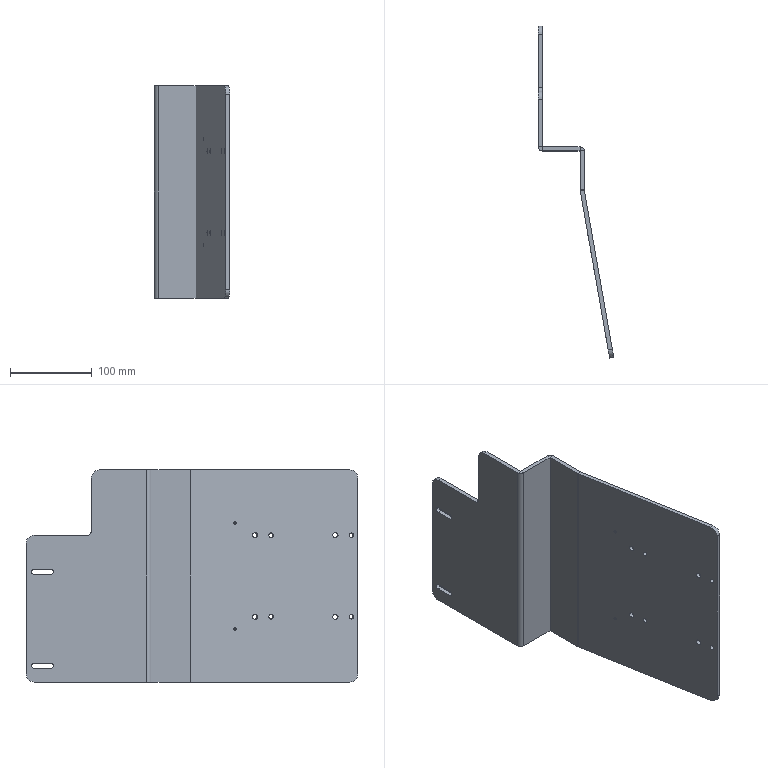Part | STEP file | monitor mounting plate | 1 solid | 68 faces | box 92.213 x 406.803 x 260 mm | volume 560601 mm3 | cylinder 38 | plane 30 | commonest cylinder face diameters 6.5 x14 5.5 x8 20 x5 3.3 x4 0.1 x3 10.1 x3